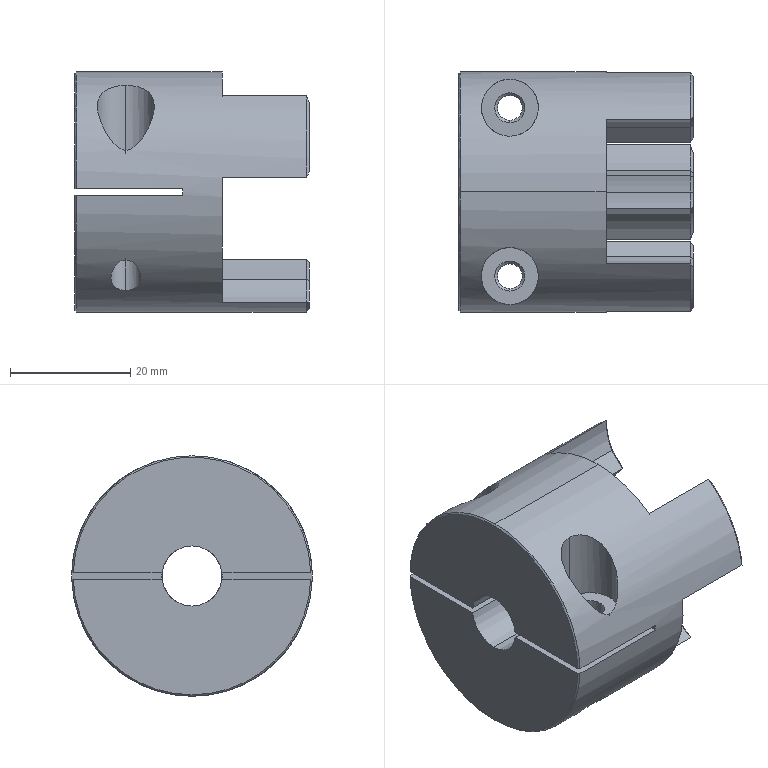Part | STEP file | L_CPJC40_10 | 1 solid | 80 faces | box 39 x 40 x 40 mm | volume 29913 mm3 | cylinder 30 | plane 26 | cone 24 | commonest cylinder face diameters 5 x8 19.758 x6 4.134 x4 9.5 x4 23 x4 10 x2